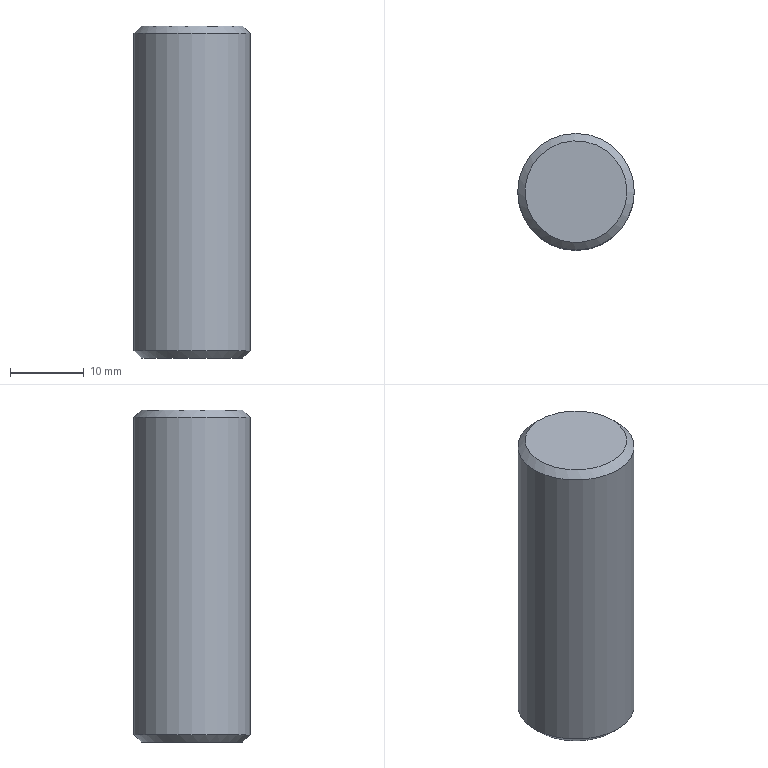Part | NX | features DATUM_CSYS 2, CHAMFER 1, EXTRUDE 1, SKETCH 1 | 1 solid | 5 faces | box 15.8 x 15.8 x 45 mm | volume 8775 mm3 | plane 2 | cone 2 | cylinder 1 | commonest cylinder face diameters 15.8 x1
STEP:
#1=CARTESIAN_POINT('',(7.9,0.,1.));
#2=VERTEX_POINT('',#1);
#3=CARTESIAN_POINT('',(0.,0.,1.));
#4=DIRECTION('',(0.,0.,1.));
#5=DIRECTION('',(1.,0.,0.));
#6=AXIS2_PLACEMENT_3D('',#3,#4,#5);
#7=CIRCLE('',#6,7.9);
#8=EDGE_CURVE('',#2,#2,#7,.T.);
#9=ORIENTED_EDGE('',*,*,#8,.T.);
#10=EDGE_LOOP('',(#9));
#11=FACE_BOUND('',#10,.T.);
#12=CARTESIAN_POINT('',(7.9,0.,44.));
#13=VERTEX_POINT('',#12);
#14=CARTESIAN_POINT('',(0.,0.,44.));
#15=DIRECTION('',(0.,0.,1.));
#16=DIRECTION('',(1.,0.,0.));
#17=AXIS2_PLACEMENT_3D('',#14,#15,#16);
#18=CIRCLE('',#17,7.9);
#19=EDGE_CURVE('',#13,#13,#18,.F.);
#20=ORIENTED_EDGE('',*,*,#19,.T.);
#21=EDGE_LOOP('',(#20));
#22=FACE_BOUND('',#21,.T.);
#23=CARTESIAN_POINT('',(0.,0.,45.));
#24=DIRECTION('',(0.,0.,-1.));
#25=DIRECTION('',(-1.,0.,0.));
#26=AXIS2_PLACEMENT_3D('',#23,#24,#25);
#27=CYLINDRICAL_SURFACE('',#26,7.9);
#28=ADVANCED_FACE('',(#11,#22),#27,.T.);
#29=CARTESIAN_POINT('',(6.9,0.,45.));
#30=VERTEX_POINT('',#29);
#31=CARTESIAN_POINT('',(0.,0.,45.));
#32=DIRECTION('',(0.,0.,1.));
#33=DIRECTION('',(1.,0.,0.));
#34=AXIS2_PLACEMENT_3D('',#31,#32,#33);
#35=CIRCLE('',#34,6.9);
#36=EDGE_CURVE('',#30,#30,#35,.T.);
#37=ORIENTED_EDGE('',*,*,#36,.T.);
#38=EDGE_LOOP('',(#37));
#39=FACE_BOUND('',#38,.T.);
#40=CARTESIAN_POINT('',(0.,0.,45.));
#41=DIRECTION('',(0.,0.,1.));
#42=DIRECTION('',(1.,0.,0.));
#43=AXIS2_PLACEMENT_3D('',#40,#41,#42);
#44=PLANE('',#43);
#45=ADVANCED_FACE('',(#39),#44,.T.);
#46=CARTESIAN_POINT('',(6.9,0.,0.));
#47=VERTEX_POINT('',#46);
#48=CARTESIAN_POINT('',(0.,0.,0.));
#49=DIRECTION('',(0.,0.,1.));
#50=DIRECTION('',(1.,0.,0.));
#51=AXIS2_PLACEMENT_3D('',#48,#49,#50);
#52=CIRCLE('',#51,6.9);
#53=EDGE_CURVE('',#47,#47,#52,.F.);
#54=ORIENTED_EDGE('',*,*,#53,.T.);
#55=EDGE_LOOP('',(#54));
#56=FACE_BOUND('',#55,.T.);
#57=CARTESIAN_POINT('',(0.,0.,0.));
#58=DIRECTION('',(0.,0.,1.));
#59=DIRECTION('',(1.,0.,0.));
#60=AXIS2_PLACEMENT_3D('',#57,#58,#59);
#61=PLANE('',#60);
#62=ADVANCED_FACE('',(#56),#61,.F.);
#63=ORIENTED_EDGE('',*,*,#53,.F.);
#64=EDGE_LOOP('',(#63));
#65=FACE_BOUND('',#64,.T.);
#66=ORIENTED_EDGE('',*,*,#8,.F.);
#67=EDGE_LOOP('',(#66));
#68=FACE_BOUND('',#67,.T.);
#69=CARTESIAN_POINT('',(0.,0.,1.));
#70=DIRECTION('',(0.,0.,1.));
#71=DIRECTION('',(1.,0.,0.));
#72=AXIS2_PLACEMENT_3D('',#69,#70,#71);
#73=CONICAL_SURFACE('',#72,7.9,0.7854);
#74=ADVANCED_FACE('',(#65,#68),#73,.T.);
#75=ORIENTED_EDGE('',*,*,#19,.F.);
#76=EDGE_LOOP('',(#75));
#77=FACE_BOUND('',#76,.T.);
#78=ORIENTED_EDGE('',*,*,#36,.F.);
#79=EDGE_LOOP('',(#78));
#80=FACE_BOUND('',#79,.T.);
#81=CARTESIAN_POINT('',(0.,0.,45.));
#82=DIRECTION('',(0.,0.,-1.));
#83=DIRECTION('',(-1.,0.,0.));
#84=AXIS2_PLACEMENT_3D('',#81,#82,#83);
#85=CONICAL_SURFACE('',#84,6.9,0.7854);
#86=ADVANCED_FACE('',(#77,#80),#85,.T.);
#87=CLOSED_SHELL('',(#28,#45,#62,#74,#86));
#88=MANIFOLD_SOLID_BREP('',#87);
#89=(LENGTH_UNIT()NAMED_UNIT(*)SI_UNIT(.MILLI.,.METRE.));
#90=UNCERTAINTY_MEASURE_WITH_UNIT(LENGTH_MEASURE(0.00001),#89,'','');
#91=(NAMED_UNIT(*)PLANE_ANGLE_UNIT()SI_UNIT($,.RADIAN.));
#92=(NAMED_UNIT(*)SI_UNIT($,.STERADIAN.)SOLID_ANGLE_UNIT());
#93=(GEOMETRIC_REPRESENTATION_CONTEXT(3)GLOBAL_UNCERTAINTY_ASSIGNED_CONTEXT((#90))GLOBAL_UNIT_ASSIGNED_CONTEXT((#89,#91,#92))REPRESENTATION_CONTEXT('',''));
#94=ADVANCED_BREP_SHAPE_REPRESENTATION('',(#88),#93);